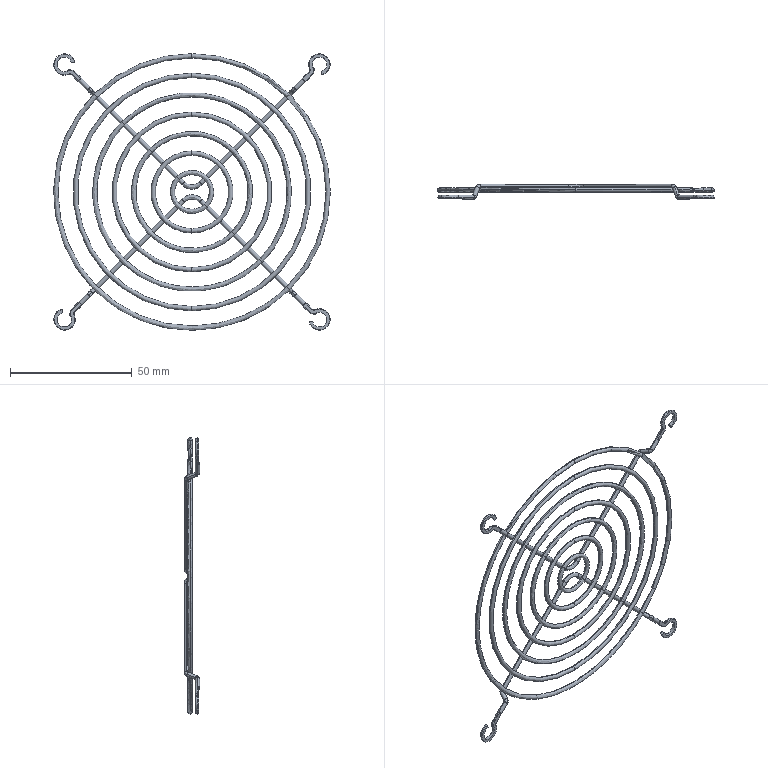Part | STEP file | 1 solid | 125 faces | box 113.8 x 6.3 x 113.8 mm | volume 4425 mm3 | spline 64 | cylinder 37 | torus 16 | plane 8 | commonest cylinder face diameters 1.8 x24 6 x9 17.441 x1 17.836 x1 18.686 x1 18.805 x1